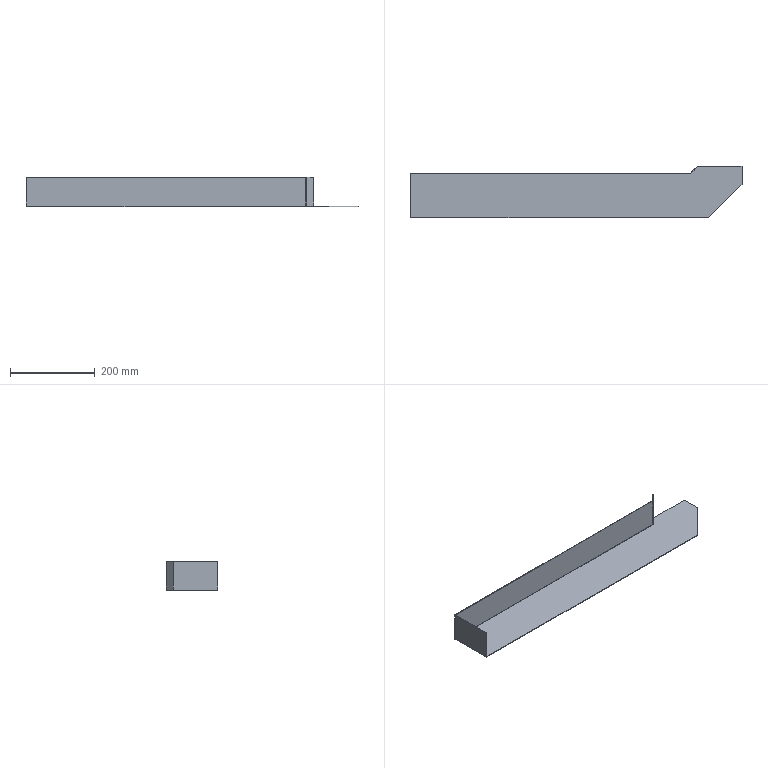Part | STEP file | Trunking 4 | 1 solid | 31 faces | box 785 x 122.735 x 70 mm | volume 203743 mm3 | plane 22 | cylinder 7 | spline 2 | commonest cylinder face diameters 0.2 x3 3.2 x3 0.15 x1
STEP:
#1=CARTESIAN_POINT('',(326.131,83.9,-1.5));
#2=VERTEX_POINT('',#1);
#3=CARTESIAN_POINT('',(-335.197,83.9,-1.5));
#4=VERTEX_POINT('',#3);
#5=CARTESIAN_POINT('',(0.,83.9,-1.5));
#6=DIRECTION('',(-1.,0.,0.));
#7=VECTOR('',#6,1000.);
#8=LINE('',#5,#7);
#9=EDGE_CURVE('',#2,#4,#8,.T.);
#10=ORIENTED_EDGE('',*,*,#9,.F.);
#11=CARTESIAN_POINT('',(343.335,101.104,-1.5));
#12=VERTEX_POINT('',#11);
#13=CARTESIAN_POINT('',(343.335,101.104,-1.5));
#14=DIRECTION('',(-0.7071,-0.7071,0.));
#15=VECTOR('',#14,1000.);
#16=LINE('',#13,#15);
#17=EDGE_CURVE('',#12,#2,#16,.T.);
#18=ORIENTED_EDGE('',*,*,#17,.F.);
#19=CARTESIAN_POINT('',(343.441,100.998,-1.5));
#20=VERTEX_POINT('',#19);
#21=CARTESIAN_POINT('',(343.335,101.104,-1.5));
#22=DIRECTION('',(-0.7071,0.7071,0.));
#23=VECTOR('',#22,1000.);
#24=LINE('',#21,#23);
#25=EDGE_CURVE('',#20,#12,#24,.T.);
#26=ORIENTED_EDGE('',*,*,#25,.F.);
#27=CARTESIAN_POINT('',(343.547,101.104,-1.5));
#28=VERTEX_POINT('',#27);
#29=CARTESIAN_POINT('',(343.494,101.051,-1.5));
#30=DIRECTION('',(0.,0.,1.));
#31=DIRECTION('',(0.,1.,0.));
#32=AXIS2_PLACEMENT_3D('',#29,#30,#31);
#33=CIRCLE('',#32,0.075);
#34=EDGE_CURVE('',#20,#28,#33,.T.);
#35=ORIENTED_EDGE('',*,*,#34,.T.);
#36=CARTESIAN_POINT('',(342.415,102.235,-1.5));
#37=VERTEX_POINT('',#36);
#38=CARTESIAN_POINT('',(342.415,102.235,-1.5));
#39=DIRECTION('',(0.7071,-0.7071,0.));
#40=VECTOR('',#39,1000.);
#41=LINE('',#38,#40);
#42=EDGE_CURVE('',#37,#28,#41,.T.);
#43=ORIENTED_EDGE('',*,*,#42,.F.);
#44=CARTESIAN_POINT('',(448.203,102.235,-1.5));
#45=VERTEX_POINT('',#44);
#46=CARTESIAN_POINT('',(0.,102.235,-1.5));
#47=DIRECTION('',(-1.,0.,0.));
#48=VECTOR('',#47,1000.);
#49=LINE('',#46,#48);
#50=EDGE_CURVE('',#45,#37,#49,.T.);
#51=ORIENTED_EDGE('',*,*,#50,.F.);
#52=CARTESIAN_POINT('',(448.203,58.328,-1.5));
#53=VERTEX_POINT('',#52);
#54=CARTESIAN_POINT('',(448.203,0.,-1.5));
#55=DIRECTION('',(0.,1.,0.));
#56=VECTOR('',#55,1000.);
#57=LINE('',#54,#56);
#58=EDGE_CURVE('',#53,#45,#57,.T.);
#59=ORIENTED_EDGE('',*,*,#58,.F.);
#60=CARTESIAN_POINT('',(369.375,-20.5,-1.5));
#61=VERTEX_POINT('',#60);
#62=CARTESIAN_POINT('',(369.375,-20.5,-1.5));
#63=DIRECTION('',(0.7071,0.7071,0.));
#64=VECTOR('',#63,1000.);
#65=LINE('',#62,#64);
#66=EDGE_CURVE('',#61,#53,#65,.T.);
#67=ORIENTED_EDGE('',*,*,#66,.F.);
#68=CARTESIAN_POINT('',(-335.197,-20.5,-1.5));
#69=VERTEX_POINT('',#68);
#70=CARTESIAN_POINT('',(0.,-20.5,-1.5));
#71=DIRECTION('',(1.,0.,0.));
#72=VECTOR('',#71,1000.);
#73=LINE('',#70,#72);
#74=EDGE_CURVE('',#69,#61,#73,.T.);
#75=ORIENTED_EDGE('',*,*,#74,.F.);
#76=CARTESIAN_POINT('',(-335.197,0.,-1.5));
#77=DIRECTION('',(0.,-1.,0.));
#78=VECTOR('',#77,1000.);
#79=LINE('',#76,#78);
#80=EDGE_CURVE('',#4,#69,#79,.T.);
#81=ORIENTED_EDGE('',*,*,#80,.F.);
#82=EDGE_LOOP('',(#10,#18,#26,#35,#43,#51,#59,#67,#75,#81));
#83=FACE_OUTER_BOUND('',#82,.T.);
#84=CARTESIAN_POINT('',(0.,0.,-1.5));
#85=DIRECTION('',(0.,0.,1.));
#86=DIRECTION('',(1.,0.,0.));
#87=AXIS2_PLACEMENT_3D('',#84,#85,#86);
#88=PLANE('',#87);
#89=ADVANCED_FACE('',(#83),#88,.F.);
#90=CARTESIAN_POINT('',(-336.794,83.9,0.));
#91=VERTEX_POINT('',#90);
#92=CARTESIAN_POINT('',(-336.797,83.9,0.1));
#93=VERTEX_POINT('',#92);
#94=CARTESIAN_POINT('',(-335.197,83.9,0.1));
#95=DIRECTION('',(0.,1.,0.));
#96=DIRECTION('',(0.,0.,1.));
#97=AXIS2_PLACEMENT_3D('',#94,#95,#96);
#98=CIRCLE('',#97,1.6);
#99=EDGE_CURVE('',#91,#93,#98,.T.);
#100=ORIENTED_EDGE('',*,*,#99,.F.);
#101=CARTESIAN_POINT('',(-335.197,83.9,0.1));
#102=DIRECTION('',(0.,-1.,0.));
#103=DIRECTION('',(0.,0.,-1.));
#104=AXIS2_PLACEMENT_3D('',#101,#102,#103);
#105=CIRCLE('',#104,1.6);
#106=EDGE_CURVE('',#91,#4,#105,.T.);
#107=ORIENTED_EDGE('',*,*,#106,.T.);
#108=ORIENTED_EDGE('',*,*,#80,.T.);
#109=CARTESIAN_POINT('',(-336.797,-20.5,0.1));
#110=VERTEX_POINT('',#109);
#111=CARTESIAN_POINT('',(-335.197,-20.5,0.1));
#112=DIRECTION('',(0.,1.,0.));
#113=DIRECTION('',(0.,0.,-1.));
#114=AXIS2_PLACEMENT_3D('',#111,#112,#113);
#115=CIRCLE('',#114,1.6);
#116=EDGE_CURVE('',#69,#110,#115,.T.);
#117=ORIENTED_EDGE('',*,*,#116,.T.);
#118=CARTESIAN_POINT('',(-336.797,-20.5,0.1));
#119=DIRECTION('',(0.,1.,0.));
#120=VECTOR('',#119,1000.);
#121=LINE('',#118,#120);
#122=EDGE_CURVE('',#110,#93,#121,.T.);
#123=ORIENTED_EDGE('',*,*,#122,.T.);
#124=EDGE_LOOP('',(#100,#107,#108,#117,#123));
#125=FACE_OUTER_BOUND('',#124,.T.);
#126=CARTESIAN_POINT('',(-335.197,-20.5,0.1));
#127=DIRECTION('',(0.,-1.,0.));
#128=DIRECTION('',(0.,0.,-1.));
#129=AXIS2_PLACEMENT_3D('',#126,#127,#128);
#130=CYLINDRICAL_SURFACE('',#129,1.6);
#131=ADVANCED_FACE('',(#125),#130,.T.);
#132=CARTESIAN_POINT('',(325.197,85.5,0.1));
#133=VERTEX_POINT('',#132);
#134=CARTESIAN_POINT('',(325.197,85.5,0.1));
#135=CARTESIAN_POINT('',(325.276,85.5,-0.1113));
#136=CARTESIAN_POINT('',(325.353,85.459,-0.3179));
#137=CARTESIAN_POINT('',(325.47,85.338,-0.6094));
#138=CARTESIAN_POINT('',(325.508,85.289,-0.7014));
#139=CARTESIAN_POINT('',(325.586,85.173,-0.8748));
#140=CARTESIAN_POINT('',(325.625,85.106,-0.957));
#141=CARTESIAN_POINT('',(325.703,84.958,-1.105));
#142=CARTESIAN_POINT('',(325.741,84.877,-1.171));
#143=CARTESIAN_POINT('',(325.819,84.703,-1.288));
#144=CARTESIAN_POINT('',(325.858,84.61,-1.338));
#145=CARTESIAN_POINT('',(325.975,84.32,-1.458));
#146=CARTESIAN_POINT('',(326.052,84.111,-1.5));
#147=CARTESIAN_POINT('',(326.131,83.9,-1.5));
#148=B_SPLINE_CURVE_WITH_KNOTS('',3,(#134,#135,#136,#137,#138,#139,#140,#141,#142,#143,#144,#145,#146,#147),.UNSPECIFIED.,.F.,.F.,(4,2,2,2,2,2,4),(0.,0.0006666,0.0009999,0.001333,0.001667,0.002,0.002666),.UNSPECIFIED.);
#149=EDGE_CURVE('',#133,#2,#148,.T.);
#150=ORIENTED_EDGE('',*,*,#149,.T.);
#151=ORIENTED_EDGE('',*,*,#9,.T.);
#152=CARTESIAN_POINT('',(-336.797,83.9,-1.5));
#153=VERTEX_POINT('',#152);
#154=CARTESIAN_POINT('',(-336.797,83.9,-1.5));
#155=DIRECTION('',(-1.,0.,0.));
#156=VECTOR('',#155,1000.);
#157=LINE('',#154,#156);
#158=EDGE_CURVE('',#4,#153,#157,.T.);
#159=ORIENTED_EDGE('',*,*,#158,.T.);
#160=CARTESIAN_POINT('',(-336.797,85.5,0.1));
#161=VERTEX_POINT('',#160);
#162=CARTESIAN_POINT('',(-336.797,83.9,0.1));
#163=DIRECTION('',(1.,0.,0.));
#164=DIRECTION('',(0.,0.,1.));
#165=AXIS2_PLACEMENT_3D('',#162,#163,#164);
#166=CIRCLE('',#165,1.6);
#167=EDGE_CURVE('',#153,#161,#166,.T.);
#168=ORIENTED_EDGE('',*,*,#167,.T.);
#169=CARTESIAN_POINT('',(-336.797,85.5,0.1));
#170=DIRECTION('',(1.,0.,0.));
#171=VECTOR('',#170,1000.);
#172=LINE('',#169,#171);
#173=EDGE_CURVE('',#161,#133,#172,.T.);
#174=ORIENTED_EDGE('',*,*,#173,.T.);
#175=EDGE_LOOP('',(#150,#151,#159,#168,#174));
#176=FACE_OUTER_BOUND('',#175,.T.);
#177=CARTESIAN_POINT('',(-336.797,83.9,0.1));
#178=DIRECTION('',(-1.,0.,0.));
#179=DIRECTION('',(0.,0.,1.));
#180=AXIS2_PLACEMENT_3D('',#177,#178,#179);
#181=CYLINDRICAL_SURFACE('',#180,1.6);
#182=ADVANCED_FACE('',(#176),#181,.T.);
#183=CARTESIAN_POINT('',(325.659,85.691,0.1));
#184=VERTEX_POINT('',#183);
#185=CARTESIAN_POINT('',(342.203,102.235,0.1));
#186=VERTEX_POINT('',#185);
#187=CARTESIAN_POINT('',(324.999,85.031,0.1));
#188=DIRECTION('',(0.7071,0.7071,0.));
#189=VECTOR('',#188,1000.);
#190=LINE('',#187,#189);
#191=EDGE_CURVE('',#184,#186,#190,.T.);
#192=ORIENTED_EDGE('',*,*,#191,.T.);
#193=CARTESIAN_POINT('',(343.335,101.104,0.1));
#194=DIRECTION('',(-0.7071,-0.7071,0.));
#195=DIRECTION('',(0.7071,-0.7071,0.));
#196=AXIS2_PLACEMENT_3D('',#193,#194,#195);
#197=CIRCLE('',#196,1.6);
#198=EDGE_CURVE('',#186,#12,#197,.T.);
#199=ORIENTED_EDGE('',*,*,#198,.T.);
#200=ORIENTED_EDGE('',*,*,#17,.T.);
#201=CARTESIAN_POINT('',(326.131,83.9,-1.5));
#202=CARTESIAN_POINT('',(326.037,84.105,-1.5));
#203=CARTESIAN_POINT('',(325.945,84.305,-1.459));
#204=CARTESIAN_POINT('',(325.822,84.594,-1.338));
#205=CARTESIAN_POINT('',(325.784,84.687,-1.289));
#206=CARTESIAN_POINT('',(325.716,84.864,-1.173));
#207=CARTESIAN_POINT('',(325.686,84.95,-1.106));
#208=CARTESIAN_POINT('',(325.636,85.11,-0.9576));
#209=CARTESIAN_POINT('',(325.616,85.184,-0.877));
#210=CARTESIAN_POINT('',(325.589,85.321,-0.7034));
#211=CARTESIAN_POINT('',(325.581,85.384,-0.6095));
#212=CARTESIAN_POINT('',(325.579,85.551,-0.32));
#213=CARTESIAN_POINT('',(325.604,85.636,-0.1113));
#214=CARTESIAN_POINT('',(325.659,85.691,0.1));
#215=B_SPLINE_CURVE_WITH_KNOTS('',3,(#201,#202,#203,#204,#205,#206,#207,#208,#209,#210,#211,#212,#213,#214),.UNSPECIFIED.,.F.,.F.,(4,2,2,2,2,2,4),(0.,0.0006666,0.0009999,0.001333,0.001667,0.002,0.002666),.UNSPECIFIED.);
#216=EDGE_CURVE('',#2,#184,#215,.T.);
#217=ORIENTED_EDGE('',*,*,#216,.T.);
#218=EDGE_LOOP('',(#192,#199,#200,#217));
#219=FACE_OUTER_BOUND('',#218,.T.);
#220=CARTESIAN_POINT('',(326.131,83.9,0.1));
#221=DIRECTION('',(-0.7071,-0.7071,0.));
#222=DIRECTION('',(0.7071,-0.7071,0.));
#223=AXIS2_PLACEMENT_3D('',#220,#221,#222);
#224=CYLINDRICAL_SURFACE('',#223,1.6);
#225=ADVANCED_FACE('',(#219),#224,.T.);
#226=CARTESIAN_POINT('',(343.547,101.104,0.));
#227=VERTEX_POINT('',#226);
#228=CARTESIAN_POINT('',(343.547,101.104,0.));
#229=DIRECTION('',(0.,0.,1.));
#230=VECTOR('',#229,1000.);
#231=LINE('',#228,#230);
#232=EDGE_CURVE('',#28,#227,#231,.T.);
#233=ORIENTED_EDGE('',*,*,#232,.T.);
#234=CARTESIAN_POINT('',(342.415,102.235,0.));
#235=VERTEX_POINT('',#234);
#236=CARTESIAN_POINT('',(342.415,102.235,0.));
#237=DIRECTION('',(0.7071,-0.7071,0.));
#238=VECTOR('',#237,1000.);
#239=LINE('',#236,#238);
#240=EDGE_CURVE('',#235,#227,#239,.T.);
#241=ORIENTED_EDGE('',*,*,#240,.F.);
#242=CARTESIAN_POINT('',(342.415,102.235,0.));
#243=DIRECTION('',(0.,0.,-1.));
#244=VECTOR('',#243,1000.);
#245=LINE('',#242,#244);
#246=EDGE_CURVE('',#235,#37,#245,.T.);
#247=ORIENTED_EDGE('',*,*,#246,.T.);
#248=ORIENTED_EDGE('',*,*,#42,.T.);
#249=EDGE_LOOP('',(#233,#241,#247,#248));
#250=FACE_OUTER_BOUND('',#249,.T.);
#251=CARTESIAN_POINT('',(343.547,101.104,0.));
#252=DIRECTION('',(-0.7071,-0.7071,0.));
#253=DIRECTION('',(0.7071,-0.7071,0.));
#254=AXIS2_PLACEMENT_3D('',#251,#252,#253);
#255=PLANE('',#254);
#256=ADVANCED_FACE('',(#250),#255,.T.);
#257=CARTESIAN_POINT('',(448.203,102.235,0.));
#258=VERTEX_POINT('',#257);
#259=CARTESIAN_POINT('',(342.203,102.235,0.));
#260=DIRECTION('',(1.,0.,0.));
#261=VECTOR('',#260,1000.);
#262=LINE('',#259,#261);
#263=EDGE_CURVE('',#235,#258,#262,.T.);
#264=ORIENTED_EDGE('',*,*,#263,.T.);
#265=CARTESIAN_POINT('',(448.203,102.235,-1.5));
#266=DIRECTION('',(0.,0.,-1.));
#267=VECTOR('',#266,1000.);
#268=LINE('',#265,#267);
#269=EDGE_CURVE('',#258,#45,#268,.T.);
#270=ORIENTED_EDGE('',*,*,#269,.T.);
#271=ORIENTED_EDGE('',*,*,#50,.T.);
#272=ORIENTED_EDGE('',*,*,#246,.F.);
#273=EDGE_LOOP('',(#264,#270,#271,#272));
#274=FACE_OUTER_BOUND('',#273,.T.);
#275=CARTESIAN_POINT('',(342.203,102.235,-1.5));
#276=DIRECTION('',(0.,1.,0.));
#277=DIRECTION('',(0.,0.,1.));
#278=AXIS2_PLACEMENT_3D('',#275,#276,#277);
#279=PLANE('',#278);
#280=ADVANCED_FACE('',(#274),#279,.T.);
#281=ORIENTED_EDGE('',*,*,#58,.T.);
#282=ORIENTED_EDGE('',*,*,#269,.F.);
#283=CARTESIAN_POINT('',(448.203,58.328,0.));
#284=VERTEX_POINT('',#283);
#285=CARTESIAN_POINT('',(448.203,58.328,0.));
#286=DIRECTION('',(0.,-1.,0.));
#287=VECTOR('',#286,1000.);
#288=LINE('',#285,#287);
#289=EDGE_CURVE('',#258,#284,#288,.T.);
#290=ORIENTED_EDGE('',*,*,#289,.T.);
#291=CARTESIAN_POINT('',(448.203,58.328,-1.5));
#292=DIRECTION('',(0.,0.,-1.));
#293=VECTOR('',#292,1000.);
#294=LINE('',#291,#293);
#295=EDGE_CURVE('',#284,#53,#294,.T.);
#296=ORIENTED_EDGE('',*,*,#295,.T.);
#297=EDGE_LOOP('',(#281,#282,#290,#296));
#298=FACE_OUTER_BOUND('',#297,.T.);
#299=CARTESIAN_POINT('',(448.203,58.328,-1.5));
#300=DIRECTION('',(1.,0.,0.));
#301=DIRECTION('',(0.,0.,-1.));
#302=AXIS2_PLACEMENT_3D('',#299,#300,#301);
#303=PLANE('',#302);
#304=ADVANCED_FACE('',(#298),#303,.T.);
#305=ORIENTED_EDGE('',*,*,#66,.T.);
#306=ORIENTED_EDGE('',*,*,#295,.F.);
#307=CARTESIAN_POINT('',(369.375,-20.5,0.));
#308=VERTEX_POINT('',#307);
#309=CARTESIAN_POINT('',(369.375,-20.5,0.));
#310=DIRECTION('',(-0.7071,-0.7071,0.));
#311=VECTOR('',#310,1000.);
#312=LINE('',#309,#311);
#313=EDGE_CURVE('',#284,#308,#312,.T.);
#314=ORIENTED_EDGE('',*,*,#313,.T.);
#315=CARTESIAN_POINT('',(369.375,-20.5,-1.5));
#316=DIRECTION('',(0.,0.,-1.));
#317=VECTOR('',#316,1000.);
#318=LINE('',#315,#317);
#319=EDGE_CURVE('',#308,#61,#318,.T.);
#320=ORIENTED_EDGE('',*,*,#319,.T.);
#321=EDGE_LOOP('',(#305,#306,#314,#320));
#322=FACE_OUTER_BOUND('',#321,.T.);
#323=CARTESIAN_POINT('',(369.375,-20.5,-1.5));
#324=DIRECTION('',(0.7071,-0.7071,0.));
#325=DIRECTION('',(0.7071,0.7071,0.));
#326=AXIS2_PLACEMENT_3D('',#323,#324,#325);
#327=PLANE('',#326);
#328=ADVANCED_FACE('',(#322),#327,.T.);
#329=ORIENTED_EDGE('',*,*,#74,.T.);
#330=ORIENTED_EDGE('',*,*,#319,.F.);
#331=CARTESIAN_POINT('',(-335.197,-20.5,0.));
#332=VERTEX_POINT('',#331);
#333=CARTESIAN_POINT('',(-336.797,-20.5,0.));
#334=DIRECTION('',(-1.,0.,0.));
#335=VECTOR('',#334,1000.);
#336=LINE('',#333,#335);
#337=EDGE_CURVE('',#308,#332,#336,.T.);
#338=ORIENTED_EDGE('',*,*,#337,.T.);
#339=CARTESIAN_POINT('',(-335.297,-20.5,0.1));
#340=VERTEX_POINT('',#339);
#341=CARTESIAN_POINT('',(-335.197,-20.5,0.1));
#342=DIRECTION('',(0.,1.,0.));
#343=DIRECTION('',(0.,0.,-1.));
#344=AXIS2_PLACEMENT_3D('',#341,#342,#343);
#345=CIRCLE('',#344,0.1);
#346=EDGE_CURVE('',#332,#340,#345,.T.);
#347=ORIENTED_EDGE('',*,*,#346,.T.);
#348=CARTESIAN_POINT('',(-335.297,-20.5,68.5));
#349=VERTEX_POINT('',#348);
#350=CARTESIAN_POINT('',(-335.297,-20.5,68.5));
#351=DIRECTION('',(0.,0.,-1.));
#352=VECTOR('',#351,1000.);
#353=LINE('',#350,#352);
#354=EDGE_CURVE('',#349,#340,#353,.T.);
#355=ORIENTED_EDGE('',*,*,#354,.F.);
#356=CARTESIAN_POINT('',(-336.797,-20.5,68.5));
#357=VERTEX_POINT('',#356);
#358=CARTESIAN_POINT('',(-336.797,-20.5,68.5));
#359=DIRECTION('',(1.,0.,0.));
#360=VECTOR('',#359,1000.);
#361=LINE('',#358,#360);
#362=EDGE_CURVE('',#357,#349,#361,.T.);
#363=ORIENTED_EDGE('',*,*,#362,.F.);
#364=CARTESIAN_POINT('',(-336.797,-20.5,0.));
#365=DIRECTION('',(0.,0.,-1.));
#366=VECTOR('',#365,1000.);
#367=LINE('',#364,#366);
#368=EDGE_CURVE('',#357,#110,#367,.T.);
#369=ORIENTED_EDGE('',*,*,#368,.T.);
#370=ORIENTED_EDGE('',*,*,#116,.F.);
#371=EDGE_LOOP('',(#329,#330,#338,#347,#355,#363,#369,#370));
#372=FACE_OUTER_BOUND('',#371,.T.);
#373=CARTESIAN_POINT('',(-336.797,-20.5,-1.5));
#374=DIRECTION('',(0.,-1.,0.));
#375=DIRECTION('',(0.,0.,-1.));
#376=AXIS2_PLACEMENT_3D('',#373,#374,#375);
#377=PLANE('',#376);
#378=ADVANCED_FACE('',(#372),#377,.T.);
#379=CARTESIAN_POINT('',(-336.797,83.9,0.));
#380=VERTEX_POINT('',#379);
#381=CARTESIAN_POINT('',(-336.797,83.9,0.));
#382=DIRECTION('',(-1.,0.,0.));
#383=VECTOR('',#382,1000.);
#384=LINE('',#381,#383);
#385=EDGE_CURVE('',#91,#380,#384,.T.);
#386=ORIENTED_EDGE('',*,*,#385,.T.);
#387=CARTESIAN_POINT('',(-336.797,83.9,0.));
#388=DIRECTION('',(0.,0.,-1.));
#389=VECTOR('',#388,1000.);
#390=LINE('',#387,#389);
#391=EDGE_CURVE('',#380,#153,#390,.T.);
#392=ORIENTED_EDGE('',*,*,#391,.T.);
#393=ORIENTED_EDGE('',*,*,#158,.F.);
#394=ORIENTED_EDGE('',*,*,#106,.F.);
#395=EDGE_LOOP('',(#386,#392,#393,#394));
#396=FACE_OUTER_BOUND('',#395,.T.);
#397=CARTESIAN_POINT('',(-335.197,83.9,0.));
#398=DIRECTION('',(0.,-1.,0.));
#399=DIRECTION('',(1.,0.,0.));
#400=AXIS2_PLACEMENT_3D('',#397,#398,#399);
#401=PLANE('',#400);
#402=ADVANCED_FACE('',(#396),#401,.T.);
#403=ORIENTED_EDGE('',*,*,#368,.F.);
#404=CARTESIAN_POINT('',(-336.797,83.9,68.5));
#405=VERTEX_POINT('',#404);
#406=CARTESIAN_POINT('',(-336.797,0.,68.5));
#407=DIRECTION('',(0.,-1.,0.));
#408=VECTOR('',#407,1000.);
#409=LINE('',#406,#408);
#410=EDGE_CURVE('',#405,#357,#409,.T.);
#411=ORIENTED_EDGE('',*,*,#410,.F.);
#412=CARTESIAN_POINT('',(-336.797,83.9,0.));
#413=DIRECTION('',(0.,0.,1.));
#414=VECTOR('',#413,1000.);
#415=LINE('',#412,#414);
#416=EDGE_CURVE('',#93,#405,#415,.T.);
#417=ORIENTED_EDGE('',*,*,#416,.F.);
#418=ORIENTED_EDGE('',*,*,#122,.F.);
#419=EDGE_LOOP('',(#403,#411,#417,#418));
#420=FACE_OUTER_BOUND('',#419,.T.);
#421=CARTESIAN_POINT('',(-336.797,0.,0.));
#422=DIRECTION('',(1.,0.,0.));
#423=DIRECTION('',(0.,0.,-1.));
#424=AXIS2_PLACEMENT_3D('',#421,#422,#423);
#425=PLANE('',#424);
#426=ADVANCED_FACE('',(#420),#425,.F.);
#427=CARTESIAN_POINT('',(325.197,84.,0.1));
#428=VERTEX_POINT('',#427);
#429=CARTESIAN_POINT('',(326.131,83.9,0.));
#430=VERTEX_POINT('',#429);
#431=CARTESIAN_POINT('',(325.197,84.,0.1));
#432=CARTESIAN_POINT('',(325.353,84.,0.07382));
#433=CARTESIAN_POINT('',(325.509,83.989,0.0478));
#434=CARTESIAN_POINT('',(325.82,83.952,0.01078));
#435=CARTESIAN_POINT('',(325.975,83.926,0.));
#436=CARTESIAN_POINT('',(326.131,83.9,0.));
#437=B_SPLINE_CURVE_WITH_KNOTS('',3,(#431,#432,#433,#434,#435,#436),.UNSPECIFIED.,.F.,.F.,(4,2,4),(0.,0.5,1.),.UNSPECIFIED.);
#438=EDGE_CURVE('',#428,#430,#437,.T.);
#439=ORIENTED_EDGE('',*,*,#438,.T.);
#440=CARTESIAN_POINT('',(326.131,83.9,-0.7575));
#441=DIRECTION('',(0.,0.,1.));
#442=VECTOR('',#441,1000.);
#443=LINE('',#440,#442);
#444=EDGE_CURVE('',#2,#430,#443,.T.);
#445=ORIENTED_EDGE('',*,*,#444,.F.);
#446=ORIENTED_EDGE('',*,*,#149,.F.);
#447=CARTESIAN_POINT('',(325.197,84.,0.1));
#448=DIRECTION('',(0.,1.,0.));
#449=VECTOR('',#448,1000.);
#450=LINE('',#447,#449);
#451=EDGE_CURVE('',#428,#133,#450,.T.);
#452=ORIENTED_EDGE('',*,*,#451,.F.);
#453=EDGE_LOOP('',(#439,#445,#446,#452));
#454=FACE_OUTER_BOUND('',#453,.T.);
#455=CARTESIAN_POINT('',(326.131,83.9,-1.515));
#456=CARTESIAN_POINT('',(326.053,84.111,-1.515));
#457=CARTESIAN_POINT('',(325.975,84.323,-1.473));
#458=CARTESIAN_POINT('',(325.82,84.713,-1.311));
#459=CARTESIAN_POINT('',(325.742,84.892,-1.191));
#460=CARTESIAN_POINT('',(325.586,85.191,-0.8925));
#461=CARTESIAN_POINT('',(325.509,85.311,-0.7133));
#462=CARTESIAN_POINT('',(325.353,85.473,-0.3227));
#463=CARTESIAN_POINT('',(325.275,85.515,-0.1114));
#464=CARTESIAN_POINT('',(325.197,85.515,0.1));
#465=CARTESIAN_POINT('',(326.131,83.9,-1.5));
#466=CARTESIAN_POINT('',(326.053,84.109,-1.5));
#467=CARTESIAN_POINT('',(325.975,84.319,-1.458));
#468=CARTESIAN_POINT('',(325.82,84.706,-1.298));
#469=CARTESIAN_POINT('',(325.742,84.883,-1.179));
#470=CARTESIAN_POINT('',(325.586,85.179,-0.8833));
#471=CARTESIAN_POINT('',(325.509,85.298,-0.7058));
#472=CARTESIAN_POINT('',(325.353,85.458,-0.3188));
#473=CARTESIAN_POINT('',(325.275,85.5,-0.1095));
#474=CARTESIAN_POINT('',(325.197,85.5,0.1));
#475=CARTESIAN_POINT('',(326.131,83.9,0.));
#476=CARTESIAN_POINT('',(326.053,83.913,0.));
#477=CARTESIAN_POINT('',(325.975,83.926,0.002603));
#478=CARTESIAN_POINT('',(325.82,83.95,0.01262));
#479=CARTESIAN_POINT('',(325.742,83.961,0.02003));
#480=CARTESIAN_POINT('',(325.586,83.98,0.03855));
#481=CARTESIAN_POINT('',(325.509,83.987,0.04964));
#482=CARTESIAN_POINT('',(325.353,83.997,0.07383));
#483=CARTESIAN_POINT('',(325.275,84.,0.08691));
#484=CARTESIAN_POINT('',(325.197,84.,0.1));
#485=B_SPLINE_SURFACE_WITH_KNOTS('',1,3,((#455,#456,#457,#458,#459,#460,#461,#462,#463,#464),(#465,#466,#467,#468,#469,#470,#471,#472,#473,#474),(#475,#476,#477,#478,#479,#480,#481,#482,#483,#484)),.UNSPECIFIED.,.F.,.F.,.F.,(2,1,2),(4,2,2,2,4),(-0.01,0.,1.),(0.,0.25,0.5,0.75,1.),.UNSPECIFIED.);
#486=ADVANCED_FACE('',(#454),#485,.F.);
#487=ORIENTED_EDGE('',*,*,#173,.F.);
#488=CARTESIAN_POINT('',(-336.797,85.5,68.5));
#489=VERTEX_POINT('',#488);
#490=CARTESIAN_POINT('',(-336.797,85.5,0.));
#491=DIRECTION('',(0.,0.,-1.));
#492=VECTOR('',#491,1000.);
#493=LINE('',#490,#492);
#494=EDGE_CURVE('',#489,#161,#493,.T.);
#495=ORIENTED_EDGE('',*,*,#494,.F.);
#496=CARTESIAN_POINT('',(325.197,85.5,68.5));
#497=VERTEX_POINT('',#496);
#498=CARTESIAN_POINT('',(0.,85.5,68.5));
#499=DIRECTION('',(-1.,0.,0.));
#500=VECTOR('',#499,1000.);
#501=LINE('',#498,#500);
#502=EDGE_CURVE('',#497,#489,#501,.T.);
#503=ORIENTED_EDGE('',*,*,#502,.F.);
#504=CARTESIAN_POINT('',(325.197,85.5,0.));
#505=DIRECTION('',(0.,0.,1.));
#506=VECTOR('',#505,1000.);
#507=LINE('',#504,#506);
#508=EDGE_CURVE('',#133,#497,#507,.T.);
#509=ORIENTED_EDGE('',*,*,#508,.F.);
#510=EDGE_LOOP('',(#487,#495,#503,#509));
#511=FACE_OUTER_BOUND('',#510,.T.);
#512=CARTESIAN_POINT('',(0.,85.5,0.));
#513=DIRECTION('',(0.,-1.,0.));
#514=DIRECTION('',(0.,0.,-1.));
#515=AXIS2_PLACEMENT_3D('',#512,#513,#514);
#516=PLANE('',#515);
#517=ADVANCED_FACE('',(#511),#516,.F.);
#518=CARTESIAN_POINT('',(-336.797,84.,0.1));
#519=VERTEX_POINT('',#518);
#520=CARTESIAN_POINT('',(-336.797,83.9,0.1));
#521=DIRECTION('',(1.,0.,0.));
#522=DIRECTION('',(0.,0.,1.));
#523=AXIS2_PLACEMENT_3D('',#520,#521,#522);
#524=CIRCLE('',#523,0.1);
#525=EDGE_CURVE('',#380,#519,#524,.T.);
#526=ORIENTED_EDGE('',*,*,#525,.T.);
#527=CARTESIAN_POINT('',(-336.797,84.,68.5));
#528=VERTEX_POINT('',#527);
#529=CARTESIAN_POINT('',(-336.797,84.,68.5));
#530=DIRECTION('',(0.,0.,-1.));
#531=VECTOR('',#530,1000.);
#532=LINE('',#529,#531);
#533=EDGE_CURVE('',#528,#519,#532,.T.);
#534=ORIENTED_EDGE('',*,*,#533,.F.);
#535=CARTESIAN_POINT('',(-336.797,85.5,68.5));
#536=DIRECTION('',(0.,-1.,0.));
#537=VECTOR('',#536,1000.);
#538=LINE('',#535,#537);
#539=EDGE_CURVE('',#489,#528,#538,.T.);
#540=ORIENTED_EDGE('',*,*,#539,.F.);
#541=ORIENTED_EDGE('',*,*,#494,.T.);
#542=ORIENTED_EDGE('',*,*,#167,.F.);
#543=ORIENTED_EDGE('',*,*,#391,.F.);
#544=EDGE_LOOP('',(#526,#534,#540,#541,#542,#543));
#545=FACE_OUTER_BOUND('',#544,.T.);
#546=CARTESIAN_POINT('',(-336.797,83.9,0.1));
#547=DIRECTION('',(1.,0.,0.));
#548=DIRECTION('',(0.,0.,-1.));
#549=AXIS2_PLACEMENT_3D('',#546,#547,#548);
#550=PLANE('',#549);
#551=ADVANCED_FACE('',(#545),#550,.F.);
#552=CARTESIAN_POINT('',(343.264,101.174,0.1));
#553=VERTEX_POINT('',#552);
#554=CARTESIAN_POINT('',(343.335,101.104,0.));
#555=VERTEX_POINT('',#554);
#556=CARTESIAN_POINT('',(343.335,101.104,0.1));
#557=DIRECTION('',(-0.7071,-0.7071,0.));
#558=DIRECTION('',(0.7071,-0.7071,0.));
#559=AXIS2_PLACEMENT_3D('',#556,#557,#558);
#560=CIRCLE('',#559,0.1);
#561=EDGE_CURVE('',#553,#555,#560,.T.);
#562=ORIENTED_EDGE('',*,*,#561,.T.);
#563=CARTESIAN_POINT('',(343.441,100.998,0.));
#564=VERTEX_POINT('',#563);
#565=CARTESIAN_POINT('',(343.441,100.998,0.));
#566=DIRECTION('',(-0.7071,0.7071,0.));
#567=VECTOR('',#566,1000.);
#568=LINE('',#565,#567);
#569=EDGE_CURVE('',#564,#555,#568,.T.);
#570=ORIENTED_EDGE('',*,*,#569,.F.);
#571=CARTESIAN_POINT('',(343.441,100.998,0.));
#572=DIRECTION('',(0.,0.,-1.));
#573=VECTOR('',#572,1000.);
#574=LINE('',#571,#573);
#575=EDGE_CURVE('',#564,#20,#574,.T.);
#576=ORIENTED_EDGE('',*,*,#575,.T.);
#577=ORIENTED_EDGE('',*,*,#25,.T.);
#578=ORIENTED_EDGE('',*,*,#198,.F.);
#579=CARTESIAN_POINT('',(342.203,102.235,68.5));
#580=VERTEX_POINT('',#579);
#581=CARTESIAN_POINT('',(342.203,102.235,0.));
#582=DIRECTION('',(0.,0.,1.));
#583=VECTOR('',#582,1000.);
#584=LINE('',#581,#583);
#585=EDGE_CURVE('',#186,#580,#584,.T.);
#586=ORIENTED_EDGE('',*,*,#585,.T.);
#587=CARTESIAN_POINT('',(343.264,101.174,68.5));
#588=VERTEX_POINT('',#587);
#589=CARTESIAN_POINT('',(342.203,102.235,68.5));
#590=DIRECTION('',(0.7071,-0.7071,0.));
#591=VECTOR('',#590,1000.);
#592=LINE('',#589,#591);
#593=EDGE_CURVE('',#580,#588,#592,.T.);
#594=ORIENTED_EDGE('',*,*,#593,.T.);
#595=CARTESIAN_POINT('',(343.264,101.174,0.));
#596=DIRECTION('',(0.,0.,1.));
#597=VECTOR('',#596,1000.);
#598=LINE('',#595,#597);
#599=EDGE_CURVE('',#553,#588,#598,.T.);
#600=ORIENTED_EDGE('',*,*,#599,.F.);
#601=EDGE_LOOP('',(#562,#570,#576,#577,#578,#586,#594,#600));
#602=FACE_OUTER_BOUND('',#601,.T.);
#603=CARTESIAN_POINT('',(343.335,101.104,0.1));
#604=DIRECTION('',(0.7071,0.7071,0.));
#605=DIRECTION('',(-0.7071,0.7071,0.));
#606=AXIS2_PLACEMENT_3D('',#603,#604,#605);
#607=PLANE('',#606);
#608=ADVANCED_FACE('',(#602),#607,.T.);
#609=CARTESIAN_POINT('',(325.659,85.691,68.5));
#610=VERTEX_POINT('',#609);
#611=CARTESIAN_POINT('',(325.659,85.691,0.));
#612=DIRECTION('',(0.,0.,-1.));
#613=VECTOR('',#612,1000.);
#614=LINE('',#611,#613);
#615=EDGE_CURVE('',#610,#184,#614,.T.);
#616=ORIENTED_EDGE('',*,*,#615,.F.);
#617=CARTESIAN_POINT('',(119.984,-119.984,68.5));
#618=DIRECTION('',(-0.7071,-0.7071,0.));
#619=VECTOR('',#618,1000.);
#620=LINE('',#617,#619);
#621=EDGE_CURVE('',#580,#610,#620,.T.);
#622=ORIENTED_EDGE('',*,*,#621,.F.);
#623=ORIENTED_EDGE('',*,*,#585,.F.);
#624=ORIENTED_EDGE('',*,*,#191,.F.);
#625=EDGE_LOOP('',(#616,#622,#623,#624));
#626=FACE_OUTER_BOUND('',#625,.T.);
#627=CARTESIAN_POINT('',(119.984,-119.984,0.));
#628=DIRECTION('',(0.7071,-0.7071,0.));
#629=DIRECTION('',(0.7071,0.7071,0.));
#630=AXIS2_PLACEMENT_3D('',#627,#628,#629);
#631=PLANE('',#630);
#632=ADVANCED_FACE('',(#626),#631,.F.);
#633=CARTESIAN_POINT('',(326.72,84.631,0.1));
#634=VERTEX_POINT('',#633);
#635=CARTESIAN_POINT('',(326.184,85.166,0.1));
#636=DIRECTION('',(0.7071,-0.7071,0.));
#637=VECTOR('',#636,1000.);
#638=LINE('',#635,#637);
#639=EDGE_CURVE('',#184,#634,#638,.T.);
#640=ORIENTED_EDGE('',*,*,#639,.F.);
#641=ORIENTED_EDGE('',*,*,#216,.F.);
#642=ORIENTED_EDGE('',*,*,#444,.T.);
#643=CARTESIAN_POINT('',(326.131,83.9,0.));
#644=CARTESIAN_POINT('',(326.222,84.029,0.));
#645=CARTESIAN_POINT('',(326.314,84.157,0.01078));
#646=CARTESIAN_POINT('',(326.508,84.403,0.0478));
#647=CARTESIAN_POINT('',(326.61,84.521,0.07382));
#648=CARTESIAN_POINT('',(326.72,84.631,0.1));
#649=B_SPLINE_CURVE_WITH_KNOTS('',3,(#643,#644,#645,#646,#647,#648),.UNSPECIFIED.,.F.,.F.,(4,2,4),(0.,0.5,1.),.UNSPECIFIED.);
#650=EDGE_CURVE('',#430,#634,#649,.T.);
#651=ORIENTED_EDGE('',*,*,#650,.T.);
#652=EDGE_LOOP('',(#640,#641,#642,#651));
#653=FACE_OUTER_BOUND('',#652,.T.);
#654=CARTESIAN_POINT('',(325.649,85.702,0.1));
#655=CARTESIAN_POINT('',(325.594,85.647,-0.1114));
#656=CARTESIAN_POINT('',(325.569,85.562,-0.3227));
#657=CARTESIAN_POINT('',(325.573,85.338,-0.7133));
#658=CARTESIAN_POINT('',(325.603,85.198,-0.8925));
#659=CARTESIAN_POINT('',(325.704,84.877,-1.191));
#660=CARTESIAN_POINT('',(325.776,84.695,-1.311));
#661=CARTESIAN_POINT('',(325.942,84.309,-1.473));
#662=CARTESIAN_POINT('',(326.036,84.105,-1.515));
#663=CARTESIAN_POINT('',(326.131,83.9,-1.515));
#664=CARTESIAN_POINT('',(325.659,85.691,0.1));
#665=CARTESIAN_POINT('',(325.604,85.636,-0.1095));
#666=CARTESIAN_POINT('',(325.579,85.552,-0.3188));
#667=CARTESIAN_POINT('',(325.582,85.329,-0.7058));
#668=CARTESIAN_POINT('',(325.611,85.19,-0.8833));
#669=CARTESIAN_POINT('',(325.711,84.87,-1.179));
#670=CARTESIAN_POINT('',(325.781,84.69,-1.298));
#671=CARTESIAN_POINT('',(325.945,84.306,-1.458));
#672=CARTESIAN_POINT('',(326.038,84.103,-1.5));
#673=CARTESIAN_POINT('',(326.131,83.9,-1.5));
#674=CARTESIAN_POINT('',(326.72,84.631,0.1));
#675=CARTESIAN_POINT('',(326.665,84.576,0.08691));
#676=CARTESIAN_POINT('',(326.612,84.519,0.07383));
#677=CARTESIAN_POINT('',(326.509,84.402,0.04964));
#678=CARTESIAN_POINT('',(326.459,84.342,0.03855));
#679=CARTESIAN_POINT('',(326.362,84.218,0.02003));
#680=CARTESIAN_POINT('',(326.315,84.156,0.01262));
#681=CARTESIAN_POINT('',(326.222,84.029,0.002603));
#682=CARTESIAN_POINT('',(326.177,83.964,0.));
#683=CARTESIAN_POINT('',(326.131,83.9,0.));
#684=B_SPLINE_SURFACE_WITH_KNOTS('',1,3,((#654,#655,#656,#657,#658,#659,#660,#661,#662,#663),(#664,#665,#666,#667,#668,#669,#670,#671,#672,#673),(#674,#675,#676,#677,#678,#679,#680,#681,#682,#683)),.UNSPECIFIED.,.F.,.F.,.F.,(2,1,2),(4,2,2,2,4),(-0.01,0.,1.),(0.,0.25,0.5,0.75,1.),.UNSPECIFIED.);
#685=ADVANCED_FACE('',(#653),#684,.F.);
#686=ORIENTED_EDGE('',*,*,#34,.F.);
#687=ORIENTED_EDGE('',*,*,#575,.F.);
#688=CARTESIAN_POINT('',(343.494,101.051,0.));
#689=DIRECTION('',(0.,0.,-1.));
#690=DIRECTION('',(0.,1.,0.));
#691=AXIS2_PLACEMENT_3D('',#688,#689,#690);
#692=CIRCLE('',#691,0.075);
#693=EDGE_CURVE('',#227,#564,#692,.T.);
#694=ORIENTED_EDGE('',*,*,#693,.F.);
#695=ORIENTED_EDGE('',*,*,#232,.F.);
#696=EDGE_LOOP('',(#686,#687,#694,#695));
#697=FACE_OUTER_BOUND('',#696,.T.);
#698=CARTESIAN_POINT('',(343.494,101.051,0.));
#699=DIRECTION('',(0.,0.,-1.));
#700=DIRECTION('',(0.,1.,0.));
#701=AXIS2_PLACEMENT_3D('',#698,#699,#700);
#702=CYLINDRICAL_SURFACE('',#701,0.075);
#703=ADVANCED_FACE('',(#697),#702,.F.);
#704=ORIENTED_EDGE('',*,*,#569,.T.);
#705=CARTESIAN_POINT('',(343.335,101.104,0.));
#706=DIRECTION('',(-0.7071,-0.7071,0.));
#707=VECTOR('',#706,1000.);
#708=LINE('',#705,#707);
#709=EDGE_CURVE('',#555,#430,#708,.T.);
#710=ORIENTED_EDGE('',*,*,#709,.T.);
#711=CARTESIAN_POINT('',(-335.197,83.9,0.));
#712=VERTEX_POINT('',#711);
#713=CARTESIAN_POINT('',(0.,83.9,0.));
#714=DIRECTION('',(-1.,0.,0.));
#715=VECTOR('',#714,1000.);
#716=LINE('',#713,#715);
#717=EDGE_CURVE('',#430,#712,#716,.T.);
#718=ORIENTED_EDGE('',*,*,#717,.T.);
#719=CARTESIAN_POINT('',(-335.197,0.,0.));
#720=DIRECTION('',(0.,-1.,0.));
#721=VECTOR('',#720,1000.);
#722=LINE('',#719,#721);
#723=EDGE_CURVE('',#712,#332,#722,.T.);
#724=ORIENTED_EDGE('',*,*,#723,.T.);
#725=ORIENTED_EDGE('',*,*,#337,.F.);
#726=ORIENTED_EDGE('',*,*,#313,.F.);
#727=ORIENTED_EDGE('',*,*,#289,.F.);
#728=ORIENTED_EDGE('',*,*,#263,.F.);
#729=ORIENTED_EDGE('',*,*,#240,.T.);
#730=ORIENTED_EDGE('',*,*,#693,.T.);
#731=EDGE_LOOP('',(#704,#710,#718,#724,#725,#726,#727,#728,#729,#730));
#732=FACE_OUTER_BOUND('',#731,.T.);
#733=CARTESIAN_POINT('',(0.,0.,0.));
#734=DIRECTION('',(0.,0.,1.));
#735=DIRECTION('',(1.,0.,0.));
#736=AXIS2_PLACEMENT_3D('',#733,#734,#735);
#737=PLANE('',#736);
#738=ADVANCED_FACE('',(#732),#737,.T.);
#739=CARTESIAN_POINT('',(-335.297,83.9,68.5));
#740=VERTEX_POINT('',#739);
#741=CARTESIAN_POINT('',(-336.797,83.9,68.5));
#742=DIRECTION('',(1.,0.,0.));
#743=VECTOR('',#742,1000.);
#744=LINE('',#741,#743);
#745=EDGE_CURVE('',#405,#740,#744,.T.);
#746=ORIENTED_EDGE('',*,*,#745,.F.);
#747=ORIENTED_EDGE('',*,*,#410,.T.);
#748=ORIENTED_EDGE('',*,*,#362,.T.);
#749=CARTESIAN_POINT('',(-335.297,83.9,68.5));
#750=DIRECTION('',(0.,-1.,0.));
#751=VECTOR('',#750,1000.);
#752=LINE('',#749,#751);
#753=EDGE_CURVE('',#740,#349,#752,.T.);
#754=ORIENTED_EDGE('',*,*,#753,.F.);
#755=EDGE_LOOP('',(#746,#747,#748,#754));
#756=FACE_OUTER_BOUND('',#755,.T.);
#757=CARTESIAN_POINT('',(-336.797,83.9,68.5));
#758=DIRECTION('',(0.,0.,-1.));
#759=DIRECTION('',(-1.,0.,0.));
#760=AXIS2_PLACEMENT_3D('',#757,#758,#759);
#761=PLANE('',#760);
#762=ADVANCED_FACE('',(#756),#761,.F.);
#763=ORIENTED_EDGE('',*,*,#416,.T.);
#764=ORIENTED_EDGE('',*,*,#745,.T.);
#765=CARTESIAN_POINT('',(-335.297,83.9,0.1));
#766=VERTEX_POINT('',#765);
#767=CARTESIAN_POINT('',(-335.297,83.9,0.));
#768=DIRECTION('',(0.,0.,1.));
#769=VECTOR('',#768,1000.);
#770=LINE('',#767,#769);
#771=EDGE_CURVE('',#766,#740,#770,.T.);
#772=ORIENTED_EDGE('',*,*,#771,.F.);
#773=CARTESIAN_POINT('',(-335.197,83.9,0.1));
#774=DIRECTION('',(0.,-1.,0.));
#775=DIRECTION('',(0.,0.,-1.));
#776=AXIS2_PLACEMENT_3D('',#773,#774,#775);
#777=CIRCLE('',#776,0.1);
#778=EDGE_CURVE('',#766,#712,#777,.T.);
#779=ORIENTED_EDGE('',*,*,#778,.T.);
#780=CARTESIAN_POINT('',(-336.797,83.9,0.));
#781=DIRECTION('',(-1.,0.,0.));
#782=VECTOR('',#781,1000.);
#783=LINE('',#780,#782);
#784=EDGE_CURVE('',#712,#91,#783,.T.);
#785=ORIENTED_EDGE('',*,*,#784,.T.);
#786=ORIENTED_EDGE('',*,*,#99,.T.);
#787=EDGE_LOOP('',(#763,#764,#772,#779,#785,#786));
#788=FACE_OUTER_BOUND('',#787,.T.);
#789=CARTESIAN_POINT('',(-336.797,83.9,0.));
#790=DIRECTION('',(0.,-1.,0.));
#791=DIRECTION('',(1.,0.,0.));
#792=AXIS2_PLACEMENT_3D('',#789,#790,#791);
#793=PLANE('',#792);
#794=ADVANCED_FACE('',(#788),#793,.F.);
#795=CARTESIAN_POINT('',(325.197,84.,68.5));
#796=VERTEX_POINT('',#795);
#797=CARTESIAN_POINT('',(325.197,84.,0.));
#798=DIRECTION('',(0.,0.,-1.));
#799=VECTOR('',#798,1000.);
#800=LINE('',#797,#799);
#801=EDGE_CURVE('',#796,#428,#800,.T.);
#802=ORIENTED_EDGE('',*,*,#801,.T.);
#803=ORIENTED_EDGE('',*,*,#451,.T.);
#804=ORIENTED_EDGE('',*,*,#508,.T.);
#805=CARTESIAN_POINT('',(325.197,84.,68.5));
#806=DIRECTION('',(0.,-1.,0.));
#807=VECTOR('',#806,1000.);
#808=LINE('',#805,#807);
#809=EDGE_CURVE('',#497,#796,#808,.T.);
#810=ORIENTED_EDGE('',*,*,#809,.T.);
#811=EDGE_LOOP('',(#802,#803,#804,#810));
#812=FACE_OUTER_BOUND('',#811,.T.);
#813=CARTESIAN_POINT('',(325.197,84.,0.));
#814=DIRECTION('',(1.,0.,0.));
#815=DIRECTION('',(0.,0.,-1.));
#816=AXIS2_PLACEMENT_3D('',#813,#814,#815);
#817=PLANE('',#816);
#818=ADVANCED_FACE('',(#812),#817,.T.);
#819=ORIENTED_EDGE('',*,*,#502,.T.);
#820=ORIENTED_EDGE('',*,*,#539,.T.);
#821=CARTESIAN_POINT('',(325.468,84.,68.5));
#822=DIRECTION('',(-1.,0.,0.));
#823=VECTOR('',#822,1000.);
#824=LINE('',#821,#823);
#825=EDGE_CURVE('',#796,#528,#824,.T.);
#826=ORIENTED_EDGE('',*,*,#825,.F.);
#827=ORIENTED_EDGE('',*,*,#809,.F.);
#828=EDGE_LOOP('',(#819,#820,#826,#827));
#829=FACE_OUTER_BOUND('',#828,.T.);
#830=CARTESIAN_POINT('',(325.468,85.5,68.5));
#831=DIRECTION('',(0.,0.,-1.));
#832=DIRECTION('',(0.,1.,0.));
#833=AXIS2_PLACEMENT_3D('',#830,#831,#832);
#834=PLANE('',#833);
#835=ADVANCED_FACE('',(#829),#834,.F.);
#836=ORIENTED_EDGE('',*,*,#615,.T.);
#837=ORIENTED_EDGE('',*,*,#639,.T.);
#838=CARTESIAN_POINT('',(326.72,84.631,68.5));
#839=VERTEX_POINT('',#838);
#840=CARTESIAN_POINT('',(326.72,84.631,0.));
#841=DIRECTION('',(0.,0.,-1.));
#842=VECTOR('',#841,1000.);
#843=LINE('',#840,#842);
#844=EDGE_CURVE('',#839,#634,#843,.T.);
#845=ORIENTED_EDGE('',*,*,#844,.F.);
#846=CARTESIAN_POINT('',(326.72,84.631,68.5));
#847=DIRECTION('',(0.7071,-0.7071,0.));
#848=VECTOR('',#847,1000.);
#849=LINE('',#846,#848);
#850=EDGE_CURVE('',#610,#839,#849,.T.);
#851=ORIENTED_EDGE('',*,*,#850,.F.);
#852=EDGE_LOOP('',(#836,#837,#845,#851));
#853=FACE_OUTER_BOUND('',#852,.T.);
#854=CARTESIAN_POINT('',(326.72,84.631,0.));
#855=DIRECTION('',(0.7071,0.7071,0.));
#856=DIRECTION('',(-0.7071,0.7071,0.));
#857=AXIS2_PLACEMENT_3D('',#854,#855,#856);
#858=PLANE('',#857);
#859=ADVANCED_FACE('',(#853),#858,.F.);
#860=ORIENTED_EDGE('',*,*,#850,.T.);
#861=CARTESIAN_POINT('',(343.264,101.174,68.5));
#862=DIRECTION('',(-0.7071,-0.7071,0.));
#863=VECTOR('',#862,1000.);
#864=LINE('',#861,#863);
#865=EDGE_CURVE('',#588,#839,#864,.T.);
#866=ORIENTED_EDGE('',*,*,#865,.F.);
#867=ORIENTED_EDGE('',*,*,#593,.F.);
#868=ORIENTED_EDGE('',*,*,#621,.T.);
#869=EDGE_LOOP('',(#860,#866,#867,#868));
#870=FACE_OUTER_BOUND('',#869,.T.);
#871=CARTESIAN_POINT('',(342.203,102.235,68.5));
#872=DIRECTION('',(0.,0.,-1.));
#873=DIRECTION('',(0.,1.,0.));
#874=AXIS2_PLACEMENT_3D('',#871,#872,#873);
#875=PLANE('',#874);
#876=ADVANCED_FACE('',(#870),#875,.F.);
#877=ORIENTED_EDGE('',*,*,#561,.F.);
#878=CARTESIAN_POINT('',(326.06,83.971,0.1));
#879=DIRECTION('',(0.7071,0.7071,0.));
#880=VECTOR('',#879,1000.);
#881=LINE('',#878,#880);
#882=EDGE_CURVE('',#634,#553,#881,.T.);
#883=ORIENTED_EDGE('',*,*,#882,.F.);
#884=ORIENTED_EDGE('',*,*,#650,.F.);
#885=ORIENTED_EDGE('',*,*,#709,.F.);
#886=EDGE_LOOP('',(#877,#883,#884,#885));
#887=FACE_OUTER_BOUND('',#886,.T.);
#888=CARTESIAN_POINT('',(326.131,83.9,0.1));
#889=DIRECTION('',(-0.7071,-0.7071,0.));
#890=DIRECTION('',(0.7071,-0.7071,0.));
#891=AXIS2_PLACEMENT_3D('',#888,#889,#890);
#892=CYLINDRICAL_SURFACE('',#891,0.1);
#893=ADVANCED_FACE('',(#887),#892,.F.);
#894=ORIENTED_EDGE('',*,*,#778,.F.);
#895=CARTESIAN_POINT('',(-335.297,-20.5,0.1));
#896=DIRECTION('',(0.,1.,0.));
#897=VECTOR('',#896,1000.);
#898=LINE('',#895,#897);
#899=EDGE_CURVE('',#340,#766,#898,.T.);
#900=ORIENTED_EDGE('',*,*,#899,.F.);
#901=ORIENTED_EDGE('',*,*,#346,.F.);
#902=ORIENTED_EDGE('',*,*,#723,.F.);
#903=EDGE_LOOP('',(#894,#900,#901,#902));
#904=FACE_OUTER_BOUND('',#903,.T.);
#905=CARTESIAN_POINT('',(-335.197,-20.5,0.1));
#906=DIRECTION('',(0.,-1.,0.));
#907=DIRECTION('',(0.,0.,-1.));
#908=AXIS2_PLACEMENT_3D('',#905,#906,#907);
#909=CYLINDRICAL_SURFACE('',#908,0.1);
#910=ADVANCED_FACE('',(#904),#909,.F.);
#911=ORIENTED_EDGE('',*,*,#784,.F.);
#912=ORIENTED_EDGE('',*,*,#717,.F.);
#913=ORIENTED_EDGE('',*,*,#438,.F.);
#914=CARTESIAN_POINT('',(-336.797,84.,0.1));
#915=DIRECTION('',(1.,0.,0.));
#916=VECTOR('',#915,1000.);
#917=LINE('',#914,#916);
#918=EDGE_CURVE('',#519,#428,#917,.T.);
#919=ORIENTED_EDGE('',*,*,#918,.F.);
#920=ORIENTED_EDGE('',*,*,#525,.F.);
#921=ORIENTED_EDGE('',*,*,#385,.F.);
#922=EDGE_LOOP('',(#911,#912,#913,#919,#920,#921));
#923=FACE_OUTER_BOUND('',#922,.T.);
#924=CARTESIAN_POINT('',(-336.797,83.9,0.1));
#925=DIRECTION('',(-1.,0.,0.));
#926=DIRECTION('',(0.,0.,1.));
#927=AXIS2_PLACEMENT_3D('',#924,#925,#926);
#928=CYLINDRICAL_SURFACE('',#927,0.1);
#929=ADVANCED_FACE('',(#923),#928,.F.);
#930=ORIENTED_EDGE('',*,*,#771,.T.);
#931=ORIENTED_EDGE('',*,*,#753,.T.);
#932=ORIENTED_EDGE('',*,*,#354,.T.);
#933=ORIENTED_EDGE('',*,*,#899,.T.);
#934=EDGE_LOOP('',(#930,#931,#932,#933));
#935=FACE_OUTER_BOUND('',#934,.T.);
#936=CARTESIAN_POINT('',(-335.297,0.,0.));
#937=DIRECTION('',(1.,0.,0.));
#938=DIRECTION('',(0.,0.,-1.));
#939=AXIS2_PLACEMENT_3D('',#936,#937,#938);
#940=PLANE('',#939);
#941=ADVANCED_FACE('',(#935),#940,.T.);
#942=ORIENTED_EDGE('',*,*,#825,.T.);
#943=ORIENTED_EDGE('',*,*,#533,.T.);
#944=ORIENTED_EDGE('',*,*,#918,.T.);
#945=ORIENTED_EDGE('',*,*,#801,.F.);
#946=EDGE_LOOP('',(#942,#943,#944,#945));
#947=FACE_OUTER_BOUND('',#946,.T.);
#948=CARTESIAN_POINT('',(0.,84.,0.));
#949=DIRECTION('',(0.,-1.,0.));
#950=DIRECTION('',(0.,0.,-1.));
#951=AXIS2_PLACEMENT_3D('',#948,#949,#950);
#952=PLANE('',#951);
#953=ADVANCED_FACE('',(#947),#952,.T.);
#954=ORIENTED_EDGE('',*,*,#599,.T.);
#955=ORIENTED_EDGE('',*,*,#865,.T.);
#956=ORIENTED_EDGE('',*,*,#844,.T.);
#957=ORIENTED_EDGE('',*,*,#882,.T.);
#958=EDGE_LOOP('',(#954,#955,#956,#957));
#959=FACE_OUTER_BOUND('',#958,.T.);
#960=CARTESIAN_POINT('',(121.045,-121.045,0.));
#961=DIRECTION('',(0.7071,-0.7071,0.));
#962=DIRECTION('',(0.7071,0.7071,0.));
#963=AXIS2_PLACEMENT_3D('',#960,#961,#962);
#964=PLANE('',#963);
#965=ADVANCED_FACE('',(#959),#964,.T.);
#966=CLOSED_SHELL('',(#89,#131,#182,#225,#256,#280,#304,#328,#378,#402,#426,#486,#517,#551,#608,#632,#685,#703,#738,#762,#794,#818,#835,#859,#876,#893,#910,#929,#941,#953,#965));
#967=MANIFOLD_SOLID_BREP('',#966);
#968=CARTESIAN_POINT('',(0.,0.,0.));
#969=DIRECTION('',(0.,0.,1.));
#970=DIRECTION('',(1.,0.,0.));
#971=AXIS2_PLACEMENT_3D('',#968,#969,#970);
#972=(LENGTH_UNIT()NAMED_UNIT(*)SI_UNIT(.MILLI.,.METRE.));
#973=UNCERTAINTY_MEASURE_WITH_UNIT(LENGTH_MEASURE(0.00001),#972,'','');
#974=(NAMED_UNIT(*)PLANE_ANGLE_UNIT()SI_UNIT($,.RADIAN.));
#975=(NAMED_UNIT(*)SI_UNIT($,.STERADIAN.)SOLID_ANGLE_UNIT());
#976=(GEOMETRIC_REPRESENTATION_CONTEXT(3)GLOBAL_UNCERTAINTY_ASSIGNED_CONTEXT((#973))GLOBAL_UNIT_ASSIGNED_CONTEXT((#972,#974,#975))REPRESENTATION_CONTEXT('',''));
#977=ADVANCED_BREP_SHAPE_REPRESENTATION('',(#967,#971),#976);